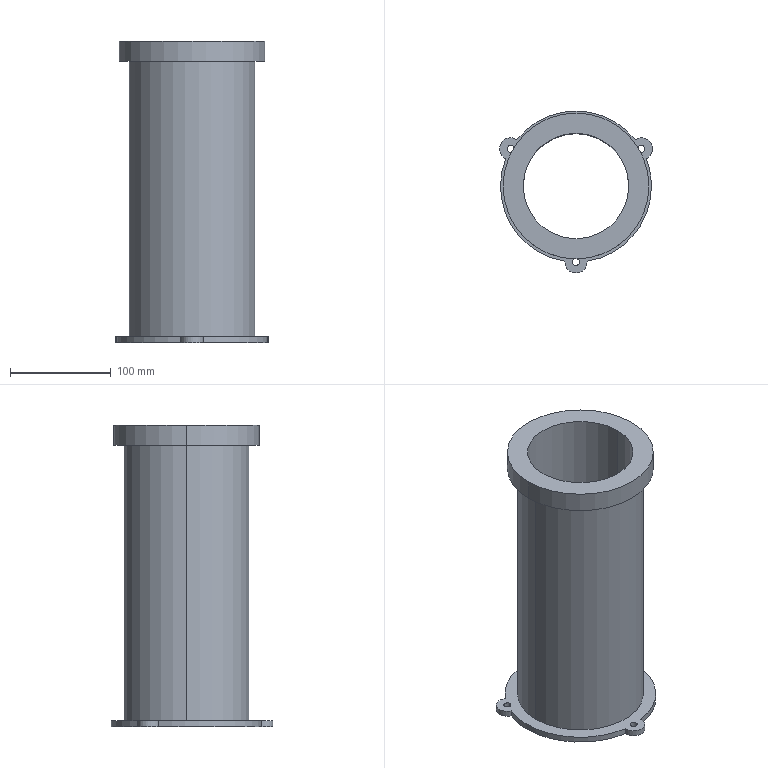Part | SolidWorks | features ICE 2, Extrusion 1 | 1 solid | 26 faces | box 151.904 x 161 x 300 mm | volume 1203905 mm3 | cylinder 22 | plane 4 | commonest cylinder face diameters 7 x6 22 x6 150 x4 105 x2 125 x2 145 x2
STEP:
#1=CARTESIAN_POINT('',(-61.452,37.5,-6.));
#2=VERTEX_POINT('',#1);
#3=CARTESIAN_POINT('',(-68.452,37.5,-6.));
#4=VERTEX_POINT('',#3);
#5=CARTESIAN_POINT('',(-64.952,37.5,-6.));
#6=DIRECTION('',(0.,0.,-1.));
#7=DIRECTION('',(-1.,0.,0.));
#8=AXIS2_PLACEMENT_3D('',#5,#6,#7);
#9=CIRCLE('',#8,3.5);
#10=EDGE_CURVE('',#2,#4,#9,.T.);
#11=ORIENTED_EDGE('',*,*,#10,.T.);
#12=CARTESIAN_POINT('',(-68.452,37.5,0.));
#13=VERTEX_POINT('',#12);
#14=CARTESIAN_POINT('',(-68.452,37.5,-6.));
#15=DIRECTION('',(0.,0.,1.));
#16=VECTOR('',#15,1000.);
#17=LINE('',#14,#16);
#18=EDGE_CURVE('',#4,#13,#17,.T.);
#19=ORIENTED_EDGE('',*,*,#18,.T.);
#20=CARTESIAN_POINT('',(-61.452,37.5,0.));
#21=VERTEX_POINT('',#20);
#22=CARTESIAN_POINT('',(-64.952,37.5,0.));
#23=DIRECTION('',(0.,0.,-1.));
#24=DIRECTION('',(-1.,0.,0.));
#25=AXIS2_PLACEMENT_3D('',#22,#23,#24);
#26=CIRCLE('',#25,3.5);
#27=EDGE_CURVE('',#21,#13,#26,.T.);
#28=ORIENTED_EDGE('',*,*,#27,.F.);
#29=CARTESIAN_POINT('',(-61.452,37.5,-6.));
#30=DIRECTION('',(0.,0.,1.));
#31=VECTOR('',#30,1000.);
#32=LINE('',#29,#31);
#33=EDGE_CURVE('',#2,#21,#32,.T.);
#34=ORIENTED_EDGE('',*,*,#33,.F.);
#35=EDGE_LOOP('',(#11,#19,#28,#34));
#36=FACE_OUTER_BOUND('',#35,.T.);
#37=CARTESIAN_POINT('',(-64.952,37.5,-6.));
#38=DIRECTION('',(0.,0.,1.));
#39=DIRECTION('',(1.,0.,0.));
#40=AXIS2_PLACEMENT_3D('',#37,#38,#39);
#41=CYLINDRICAL_SURFACE('',#40,3.5);
#42=ADVANCED_FACE('',(#36),#41,.F.);
#43=CARTESIAN_POINT('',(68.452,37.5,-6.));
#44=VERTEX_POINT('',#43);
#45=CARTESIAN_POINT('',(61.452,37.5,-6.));
#46=VERTEX_POINT('',#45);
#47=CARTESIAN_POINT('',(64.952,37.5,-6.));
#48=DIRECTION('',(0.,0.,-1.));
#49=DIRECTION('',(-1.,0.,0.));
#50=AXIS2_PLACEMENT_3D('',#47,#48,#49);
#51=CIRCLE('',#50,3.5);
#52=EDGE_CURVE('',#44,#46,#51,.T.);
#53=ORIENTED_EDGE('',*,*,#52,.T.);
#54=CARTESIAN_POINT('',(61.452,37.5,0.));
#55=VERTEX_POINT('',#54);
#56=CARTESIAN_POINT('',(61.452,37.5,-6.));
#57=DIRECTION('',(0.,0.,1.));
#58=VECTOR('',#57,1000.);
#59=LINE('',#56,#58);
#60=EDGE_CURVE('',#46,#55,#59,.T.);
#61=ORIENTED_EDGE('',*,*,#60,.T.);
#62=CARTESIAN_POINT('',(68.452,37.5,0.));
#63=VERTEX_POINT('',#62);
#64=CARTESIAN_POINT('',(64.952,37.5,0.));
#65=DIRECTION('',(0.,0.,-1.));
#66=DIRECTION('',(-1.,0.,0.));
#67=AXIS2_PLACEMENT_3D('',#64,#65,#66);
#68=CIRCLE('',#67,3.5);
#69=EDGE_CURVE('',#63,#55,#68,.T.);
#70=ORIENTED_EDGE('',*,*,#69,.F.);
#71=CARTESIAN_POINT('',(68.452,37.5,-6.));
#72=DIRECTION('',(0.,0.,1.));
#73=VECTOR('',#72,1000.);
#74=LINE('',#71,#73);
#75=EDGE_CURVE('',#44,#63,#74,.T.);
#76=ORIENTED_EDGE('',*,*,#75,.F.);
#77=EDGE_LOOP('',(#53,#61,#70,#76));
#78=FACE_OUTER_BOUND('',#77,.T.);
#79=CARTESIAN_POINT('',(64.952,37.5,-6.));
#80=DIRECTION('',(0.,0.,1.));
#81=DIRECTION('',(1.,0.,0.));
#82=AXIS2_PLACEMENT_3D('',#79,#80,#81);
#83=CYLINDRICAL_SURFACE('',#82,3.5);
#84=ADVANCED_FACE('',(#78),#83,.F.);
#85=CARTESIAN_POINT('',(3.5,-75.,-6.));
#86=VERTEX_POINT('',#85);
#87=CARTESIAN_POINT('',(-3.5,-75.,-6.));
#88=VERTEX_POINT('',#87);
#89=CARTESIAN_POINT('',(0.,-75.,-6.));
#90=DIRECTION('',(0.,0.,-1.));
#91=DIRECTION('',(-1.,0.,0.));
#92=AXIS2_PLACEMENT_3D('',#89,#90,#91);
#93=CIRCLE('',#92,3.5);
#94=EDGE_CURVE('',#86,#88,#93,.T.);
#95=ORIENTED_EDGE('',*,*,#94,.T.);
#96=CARTESIAN_POINT('',(-3.5,-75.,0.));
#97=VERTEX_POINT('',#96);
#98=CARTESIAN_POINT('',(-3.5,-75.,-6.));
#99=DIRECTION('',(0.,0.,1.));
#100=VECTOR('',#99,1000.);
#101=LINE('',#98,#100);
#102=EDGE_CURVE('',#88,#97,#101,.T.);
#103=ORIENTED_EDGE('',*,*,#102,.T.);
#104=CARTESIAN_POINT('',(3.5,-75.,0.));
#105=VERTEX_POINT('',#104);
#106=CARTESIAN_POINT('',(0.,-75.,0.));
#107=DIRECTION('',(0.,0.,-1.));
#108=DIRECTION('',(-1.,0.,0.));
#109=AXIS2_PLACEMENT_3D('',#106,#107,#108);
#110=CIRCLE('',#109,3.5);
#111=EDGE_CURVE('',#105,#97,#110,.T.);
#112=ORIENTED_EDGE('',*,*,#111,.F.);
#113=CARTESIAN_POINT('',(3.5,-75.,-6.));
#114=DIRECTION('',(0.,0.,1.));
#115=VECTOR('',#114,1000.);
#116=LINE('',#113,#115);
#117=EDGE_CURVE('',#86,#105,#116,.T.);
#118=ORIENTED_EDGE('',*,*,#117,.F.);
#119=EDGE_LOOP('',(#95,#103,#112,#118));
#120=FACE_OUTER_BOUND('',#119,.T.);
#121=CARTESIAN_POINT('',(0.,-75.,-6.));
#122=DIRECTION('',(0.,0.,1.));
#123=DIRECTION('',(1.,0.,0.));
#124=AXIS2_PLACEMENT_3D('',#121,#122,#123);
#125=CYLINDRICAL_SURFACE('',#124,3.5);
#126=ADVANCED_FACE('',(#120),#125,.F.);
#127=CARTESIAN_POINT('',(75.,0.,-6.));
#128=VERTEX_POINT('',#127);
#129=CARTESIAN_POINT('',(10.97,-74.193,-6.));
#130=VERTEX_POINT('',#129);
#131=CARTESIAN_POINT('',(0.,0.,-6.));
#132=DIRECTION('',(0.,0.,-1.));
#133=DIRECTION('',(-1.,0.,0.));
#134=AXIS2_PLACEMENT_3D('',#131,#132,#133);
#135=CIRCLE('',#134,75.);
#136=EDGE_CURVE('',#128,#130,#135,.T.);
#137=ORIENTED_EDGE('',*,*,#136,.F.);
#138=CARTESIAN_POINT('',(75.,0.,0.));
#139=VERTEX_POINT('',#138);
#140=CARTESIAN_POINT('',(75.,0.,-6.));
#141=DIRECTION('',(0.,0.,1.));
#142=VECTOR('',#141,1000.);
#143=LINE('',#140,#142);
#144=EDGE_CURVE('',#128,#139,#143,.T.);
#145=ORIENTED_EDGE('',*,*,#144,.T.);
#146=CARTESIAN_POINT('',(10.97,-74.193,0.));
#147=VERTEX_POINT('',#146);
#148=CARTESIAN_POINT('',(0.,0.,0.));
#149=DIRECTION('',(0.,0.,-1.));
#150=DIRECTION('',(-1.,0.,0.));
#151=AXIS2_PLACEMENT_3D('',#148,#149,#150);
#152=CIRCLE('',#151,75.);
#153=EDGE_CURVE('',#139,#147,#152,.T.);
#154=ORIENTED_EDGE('',*,*,#153,.T.);
#155=CARTESIAN_POINT('',(10.97,-74.193,-6.));
#156=DIRECTION('',(0.,0.,1.));
#157=VECTOR('',#156,1000.);
#158=LINE('',#155,#157);
#159=EDGE_CURVE('',#130,#147,#158,.T.);
#160=ORIENTED_EDGE('',*,*,#159,.F.);
#161=EDGE_LOOP('',(#137,#145,#154,#160));
#162=FACE_OUTER_BOUND('',#161,.T.);
#163=CARTESIAN_POINT('',(0.,0.,-6.));
#164=DIRECTION('',(0.,0.,1.));
#165=DIRECTION('',(1.,0.,0.));
#166=AXIS2_PLACEMENT_3D('',#163,#164,#165);
#167=CYLINDRICAL_SURFACE('',#166,75.);
#168=ADVANCED_FACE('',(#162),#167,.T.);
#169=CARTESIAN_POINT('',(75.952,37.5,-6.));
#170=VERTEX_POINT('',#169);
#171=CARTESIAN_POINT('',(69.739,27.596,-6.));
#172=VERTEX_POINT('',#171);
#173=CARTESIAN_POINT('',(64.952,37.5,-6.));
#174=DIRECTION('',(0.,0.,-1.));
#175=DIRECTION('',(-1.,0.,0.));
#176=AXIS2_PLACEMENT_3D('',#173,#174,#175);
#177=CIRCLE('',#176,11.);
#178=EDGE_CURVE('',#170,#172,#177,.T.);
#179=ORIENTED_EDGE('',*,*,#178,.F.);
#180=CARTESIAN_POINT('',(75.952,37.5,0.));
#181=VERTEX_POINT('',#180);
#182=CARTESIAN_POINT('',(75.952,37.5,-6.));
#183=DIRECTION('',(0.,0.,1.));
#184=VECTOR('',#183,1000.);
#185=LINE('',#182,#184);
#186=EDGE_CURVE('',#170,#181,#185,.T.);
#187=ORIENTED_EDGE('',*,*,#186,.T.);
#188=CARTESIAN_POINT('',(69.739,27.596,0.));
#189=VERTEX_POINT('',#188);
#190=CARTESIAN_POINT('',(64.952,37.5,0.));
#191=DIRECTION('',(0.,0.,-1.));
#192=DIRECTION('',(-1.,0.,0.));
#193=AXIS2_PLACEMENT_3D('',#190,#191,#192);
#194=CIRCLE('',#193,11.);
#195=EDGE_CURVE('',#181,#189,#194,.T.);
#196=ORIENTED_EDGE('',*,*,#195,.T.);
#197=CARTESIAN_POINT('',(69.739,27.596,-6.));
#198=DIRECTION('',(0.,0.,1.));
#199=VECTOR('',#198,1000.);
#200=LINE('',#197,#199);
#201=EDGE_CURVE('',#172,#189,#200,.T.);
#202=ORIENTED_EDGE('',*,*,#201,.F.);
#203=EDGE_LOOP('',(#179,#187,#196,#202));
#204=FACE_OUTER_BOUND('',#203,.T.);
#205=CARTESIAN_POINT('',(64.952,37.5,-6.));
#206=DIRECTION('',(0.,0.,1.));
#207=DIRECTION('',(1.,0.,0.));
#208=AXIS2_PLACEMENT_3D('',#205,#206,#207);
#209=CYLINDRICAL_SURFACE('',#208,11.);
#210=ADVANCED_FACE('',(#204),#209,.T.);
#211=CARTESIAN_POINT('',(-11.,-75.,-6.));
#212=VERTEX_POINT('',#211);
#213=CARTESIAN_POINT('',(-10.97,-74.193,-6.));
#214=VERTEX_POINT('',#213);
#215=CARTESIAN_POINT('',(0.,-75.,-6.));
#216=DIRECTION('',(0.,0.,-1.));
#217=DIRECTION('',(-1.,0.,0.));
#218=AXIS2_PLACEMENT_3D('',#215,#216,#217);
#219=CIRCLE('',#218,11.);
#220=EDGE_CURVE('',#212,#214,#219,.T.);
#221=ORIENTED_EDGE('',*,*,#220,.F.);
#222=CARTESIAN_POINT('',(-11.,-75.,0.));
#223=VERTEX_POINT('',#222);
#224=CARTESIAN_POINT('',(-11.,-75.,-6.));
#225=DIRECTION('',(0.,0.,1.));
#226=VECTOR('',#225,1000.);
#227=LINE('',#224,#226);
#228=EDGE_CURVE('',#212,#223,#227,.T.);
#229=ORIENTED_EDGE('',*,*,#228,.T.);
#230=CARTESIAN_POINT('',(-10.97,-74.193,0.));
#231=VERTEX_POINT('',#230);
#232=CARTESIAN_POINT('',(0.,-75.,0.));
#233=DIRECTION('',(0.,0.,-1.));
#234=DIRECTION('',(-1.,0.,0.));
#235=AXIS2_PLACEMENT_3D('',#232,#233,#234);
#236=CIRCLE('',#235,11.);
#237=EDGE_CURVE('',#223,#231,#236,.T.);
#238=ORIENTED_EDGE('',*,*,#237,.T.);
#239=CARTESIAN_POINT('',(-10.97,-74.193,-6.));
#240=DIRECTION('',(0.,0.,1.));
#241=VECTOR('',#240,1000.);
#242=LINE('',#239,#241);
#243=EDGE_CURVE('',#214,#231,#242,.T.);
#244=ORIENTED_EDGE('',*,*,#243,.F.);
#245=EDGE_LOOP('',(#221,#229,#238,#244));
#246=FACE_OUTER_BOUND('',#245,.T.);
#247=CARTESIAN_POINT('',(0.,-75.,-6.));
#248=DIRECTION('',(0.,0.,1.));
#249=DIRECTION('',(1.,0.,0.));
#250=AXIS2_PLACEMENT_3D('',#247,#248,#249);
#251=CYLINDRICAL_SURFACE('',#250,11.);
#252=ADVANCED_FACE('',(#246),#251,.T.);
#253=ORIENTED_EDGE('',*,*,#228,.F.);
#254=CARTESIAN_POINT('',(11.,-75.,-6.));
#255=VERTEX_POINT('',#254);
#256=CARTESIAN_POINT('',(0.,-75.,-6.));
#257=DIRECTION('',(0.,0.,-1.));
#258=DIRECTION('',(-1.,0.,0.));
#259=AXIS2_PLACEMENT_3D('',#256,#257,#258);
#260=CIRCLE('',#259,11.);
#261=EDGE_CURVE('',#255,#212,#260,.T.);
#262=ORIENTED_EDGE('',*,*,#261,.F.);
#263=CARTESIAN_POINT('',(11.,-75.,0.));
#264=VERTEX_POINT('',#263);
#265=CARTESIAN_POINT('',(11.,-75.,-6.));
#266=DIRECTION('',(0.,0.,1.));
#267=VECTOR('',#266,1000.);
#268=LINE('',#265,#267);
#269=EDGE_CURVE('',#255,#264,#268,.T.);
#270=ORIENTED_EDGE('',*,*,#269,.T.);
#271=CARTESIAN_POINT('',(0.,-75.,0.));
#272=DIRECTION('',(0.,0.,-1.));
#273=DIRECTION('',(-1.,0.,0.));
#274=AXIS2_PLACEMENT_3D('',#271,#272,#273);
#275=CIRCLE('',#274,11.);
#276=EDGE_CURVE('',#264,#223,#275,.T.);
#277=ORIENTED_EDGE('',*,*,#276,.T.);
#278=EDGE_LOOP('',(#253,#262,#270,#277));
#279=FACE_OUTER_BOUND('',#278,.T.);
#280=CARTESIAN_POINT('',(0.,-75.,-6.));
#281=DIRECTION('',(0.,0.,1.));
#282=DIRECTION('',(1.,0.,0.));
#283=AXIS2_PLACEMENT_3D('',#280,#281,#282);
#284=CYLINDRICAL_SURFACE('',#283,11.);
#285=ADVANCED_FACE('',(#279),#284,.T.);
#286=CARTESIAN_POINT('',(72.5,0.,294.));
#287=VERTEX_POINT('',#286);
#288=CARTESIAN_POINT('',(-72.5,0.,294.));
#289=VERTEX_POINT('',#288);
#290=CARTESIAN_POINT('',(0.,0.,294.));
#291=DIRECTION('',(0.,0.,1.));
#292=DIRECTION('',(1.,0.,0.));
#293=AXIS2_PLACEMENT_3D('',#290,#291,#292);
#294=CIRCLE('',#293,72.5);
#295=EDGE_CURVE('',#287,#289,#294,.T.);
#296=ORIENTED_EDGE('',*,*,#295,.F.);
#297=CARTESIAN_POINT('',(72.5,0.,274.));
#298=VERTEX_POINT('',#297);
#299=CARTESIAN_POINT('',(72.5,0.,294.));
#300=DIRECTION('',(0.,0.,-1.));
#301=VECTOR('',#300,1000.);
#302=LINE('',#299,#301);
#303=EDGE_CURVE('',#287,#298,#302,.T.);
#304=ORIENTED_EDGE('',*,*,#303,.T.);
#305=CARTESIAN_POINT('',(-72.5,0.,274.));
#306=VERTEX_POINT('',#305);
#307=CARTESIAN_POINT('',(0.,0.,274.));
#308=DIRECTION('',(0.,0.,1.));
#309=DIRECTION('',(1.,0.,0.));
#310=AXIS2_PLACEMENT_3D('',#307,#308,#309);
#311=CIRCLE('',#310,72.5);
#312=EDGE_CURVE('',#298,#306,#311,.T.);
#313=ORIENTED_EDGE('',*,*,#312,.T.);
#314=CARTESIAN_POINT('',(-72.5,0.,294.));
#315=DIRECTION('',(0.,0.,-1.));
#316=VECTOR('',#315,1000.);
#317=LINE('',#314,#316);
#318=EDGE_CURVE('',#289,#306,#317,.T.);
#319=ORIENTED_EDGE('',*,*,#318,.F.);
#320=EDGE_LOOP('',(#296,#304,#313,#319));
#321=FACE_OUTER_BOUND('',#320,.T.);
#322=CARTESIAN_POINT('',(0.,0.,294.));
#323=DIRECTION('',(0.,0.,-1.));
#324=DIRECTION('',(-1.,0.,0.));
#325=AXIS2_PLACEMENT_3D('',#322,#323,#324);
#326=CYLINDRICAL_SURFACE('',#325,72.5);
#327=ADVANCED_FACE('',(#321),#326,.T.);
#328=CARTESIAN_POINT('',(-52.5,0.,294.));
#329=VERTEX_POINT('',#328);
#330=CARTESIAN_POINT('',(52.5,0.,294.));
#331=VERTEX_POINT('',#330);
#332=CARTESIAN_POINT('',(0.,0.,294.));
#333=DIRECTION('',(0.,0.,1.));
#334=DIRECTION('',(1.,0.,0.));
#335=AXIS2_PLACEMENT_3D('',#332,#333,#334);
#336=CIRCLE('',#335,52.5);
#337=EDGE_CURVE('',#329,#331,#336,.T.);
#338=ORIENTED_EDGE('',*,*,#337,.T.);
#339=CARTESIAN_POINT('',(52.5,0.,-6.));
#340=VERTEX_POINT('',#339);
#341=CARTESIAN_POINT('',(52.5,0.,284.));
#342=DIRECTION('',(0.,0.,-1.));
#343=VECTOR('',#342,1000.);
#344=LINE('',#341,#343);
#345=EDGE_CURVE('',#331,#340,#344,.T.);
#346=ORIENTED_EDGE('',*,*,#345,.T.);
#347=CARTESIAN_POINT('',(-52.5,0.,-6.));
#348=VERTEX_POINT('',#347);
#349=CARTESIAN_POINT('',(0.,0.,-6.));
#350=DIRECTION('',(0.,0.,-1.));
#351=DIRECTION('',(-1.,0.,0.));
#352=AXIS2_PLACEMENT_3D('',#349,#350,#351);
#353=CIRCLE('',#352,52.5);
#354=EDGE_CURVE('',#340,#348,#353,.T.);
#355=ORIENTED_EDGE('',*,*,#354,.T.);
#356=CARTESIAN_POINT('',(-52.5,0.,284.));
#357=DIRECTION('',(0.,0.,-1.));
#358=VECTOR('',#357,1000.);
#359=LINE('',#356,#358);
#360=EDGE_CURVE('',#329,#348,#359,.T.);
#361=ORIENTED_EDGE('',*,*,#360,.F.);
#362=EDGE_LOOP('',(#338,#346,#355,#361));
#363=FACE_OUTER_BOUND('',#362,.T.);
#364=CARTESIAN_POINT('',(0.,0.,284.));
#365=DIRECTION('',(0.,0.,-1.));
#366=DIRECTION('',(-1.,0.,0.));
#367=AXIS2_PLACEMENT_3D('',#364,#365,#366);
#368=CYLINDRICAL_SURFACE('',#367,52.5);
#369=ADVANCED_FACE('',(#363),#368,.F.);
#370=CARTESIAN_POINT('',(62.5,0.,274.));
#371=VERTEX_POINT('',#370);
#372=CARTESIAN_POINT('',(-62.5,0.,274.));
#373=VERTEX_POINT('',#372);
#374=CARTESIAN_POINT('',(0.,0.,274.));
#375=DIRECTION('',(0.,0.,1.));
#376=DIRECTION('',(1.,0.,0.));
#377=AXIS2_PLACEMENT_3D('',#374,#375,#376);
#378=CIRCLE('',#377,62.5);
#379=EDGE_CURVE('',#371,#373,#378,.T.);
#380=ORIENTED_EDGE('',*,*,#379,.F.);
#381=CARTESIAN_POINT('',(62.5,0.,0.));
#382=VERTEX_POINT('',#381);
#383=CARTESIAN_POINT('',(62.5,0.,284.));
#384=DIRECTION('',(0.,0.,-1.));
#385=VECTOR('',#384,1000.);
#386=LINE('',#383,#385);
#387=EDGE_CURVE('',#371,#382,#386,.T.);
#388=ORIENTED_EDGE('',*,*,#387,.T.);
#389=CARTESIAN_POINT('',(-62.5,0.,0.));
#390=VERTEX_POINT('',#389);
#391=CARTESIAN_POINT('',(0.,0.,0.));
#392=DIRECTION('',(0.,0.,-1.));
#393=DIRECTION('',(-1.,0.,0.));
#394=AXIS2_PLACEMENT_3D('',#391,#392,#393);
#395=CIRCLE('',#394,62.5);
#396=EDGE_CURVE('',#390,#382,#395,.T.);
#397=ORIENTED_EDGE('',*,*,#396,.F.);
#398=CARTESIAN_POINT('',(-62.5,0.,284.));
#399=DIRECTION('',(0.,0.,-1.));
#400=VECTOR('',#399,1000.);
#401=LINE('',#398,#400);
#402=EDGE_CURVE('',#373,#390,#401,.T.);
#403=ORIENTED_EDGE('',*,*,#402,.F.);
#404=EDGE_LOOP('',(#380,#388,#397,#403));
#405=FACE_OUTER_BOUND('',#404,.T.);
#406=CARTESIAN_POINT('',(0.,0.,284.));
#407=DIRECTION('',(0.,0.,-1.));
#408=DIRECTION('',(-1.,0.,0.));
#409=AXIS2_PLACEMENT_3D('',#406,#407,#408);
#410=CYLINDRICAL_SURFACE('',#409,62.5);
#411=ADVANCED_FACE('',(#405),#410,.T.);
#412=ORIENTED_EDGE('',*,*,#387,.F.);
#413=CARTESIAN_POINT('',(0.,0.,274.));
#414=DIRECTION('',(0.,0.,1.));
#415=DIRECTION('',(1.,0.,0.));
#416=AXIS2_PLACEMENT_3D('',#413,#414,#415);
#417=CIRCLE('',#416,62.5);
#418=EDGE_CURVE('',#373,#371,#417,.T.);
#419=ORIENTED_EDGE('',*,*,#418,.F.);
#420=ORIENTED_EDGE('',*,*,#402,.T.);
#421=CARTESIAN_POINT('',(0.,0.,0.));
#422=DIRECTION('',(0.,0.,-1.));
#423=DIRECTION('',(-1.,0.,0.));
#424=AXIS2_PLACEMENT_3D('',#421,#422,#423);
#425=CIRCLE('',#424,62.5);
#426=EDGE_CURVE('',#382,#390,#425,.T.);
#427=ORIENTED_EDGE('',*,*,#426,.F.);
#428=EDGE_LOOP('',(#412,#419,#420,#427));
#429=FACE_OUTER_BOUND('',#428,.T.);
#430=CARTESIAN_POINT('',(0.,0.,284.));
#431=DIRECTION('',(0.,0.,-1.));
#432=DIRECTION('',(-1.,0.,0.));
#433=AXIS2_PLACEMENT_3D('',#430,#431,#432);
#434=CYLINDRICAL_SURFACE('',#433,62.5);
#435=ADVANCED_FACE('',(#429),#434,.T.);
#436=ORIENTED_EDGE('',*,*,#345,.F.);
#437=CARTESIAN_POINT('',(0.,0.,294.));
#438=DIRECTION('',(0.,0.,1.));
#439=DIRECTION('',(1.,0.,0.));
#440=AXIS2_PLACEMENT_3D('',#437,#438,#439);
#441=CIRCLE('',#440,52.5);
#442=EDGE_CURVE('',#331,#329,#441,.T.);
#443=ORIENTED_EDGE('',*,*,#442,.T.);
#444=ORIENTED_EDGE('',*,*,#360,.T.);
#445=CARTESIAN_POINT('',(0.,0.,-6.));
#446=DIRECTION('',(0.,0.,-1.));
#447=DIRECTION('',(-1.,0.,0.));
#448=AXIS2_PLACEMENT_3D('',#445,#446,#447);
#449=CIRCLE('',#448,52.5);
#450=EDGE_CURVE('',#348,#340,#449,.T.);
#451=ORIENTED_EDGE('',*,*,#450,.T.);
#452=EDGE_LOOP('',(#436,#443,#444,#451));
#453=FACE_OUTER_BOUND('',#452,.T.);
#454=CARTESIAN_POINT('',(0.,0.,284.));
#455=DIRECTION('',(0.,0.,-1.));
#456=DIRECTION('',(-1.,0.,0.));
#457=AXIS2_PLACEMENT_3D('',#454,#455,#456);
#458=CYLINDRICAL_SURFACE('',#457,52.5);
#459=ADVANCED_FACE('',(#453),#458,.F.);
#460=CARTESIAN_POINT('',(0.,0.,274.));
#461=DIRECTION('',(0.,0.,1.));
#462=DIRECTION('',(1.,0.,0.));
#463=AXIS2_PLACEMENT_3D('',#460,#461,#462);
#464=CIRCLE('',#463,72.5);
#465=EDGE_CURVE('',#306,#298,#464,.T.);
#466=ORIENTED_EDGE('',*,*,#465,.F.);
#467=ORIENTED_EDGE('',*,*,#312,.F.);
#468=EDGE_LOOP('',(#466,#467));
#469=FACE_OUTER_BOUND('',#468,.T.);
#470=ORIENTED_EDGE('',*,*,#418,.T.);
#471=ORIENTED_EDGE('',*,*,#379,.T.);
#472=EDGE_LOOP('',(#470,#471));
#473=FACE_BOUND('',#472,.T.);
#474=CARTESIAN_POINT('',(0.,0.,274.));
#475=DIRECTION('',(0.,0.,1.));
#476=DIRECTION('',(1.,0.,0.));
#477=AXIS2_PLACEMENT_3D('',#474,#475,#476);
#478=PLANE('',#477);
#479=ADVANCED_FACE('',(#469,#473),#478,.F.);
#480=CARTESIAN_POINT('',(0.,0.,294.));
#481=DIRECTION('',(0.,0.,1.));
#482=DIRECTION('',(1.,0.,0.));
#483=AXIS2_PLACEMENT_3D('',#480,#481,#482);
#484=CIRCLE('',#483,72.5);
#485=EDGE_CURVE('',#289,#287,#484,.T.);
#486=ORIENTED_EDGE('',*,*,#485,.T.);
#487=ORIENTED_EDGE('',*,*,#295,.T.);
#488=EDGE_LOOP('',(#486,#487));
#489=FACE_OUTER_BOUND('',#488,.T.);
#490=ORIENTED_EDGE('',*,*,#337,.F.);
#491=ORIENTED_EDGE('',*,*,#442,.F.);
#492=EDGE_LOOP('',(#490,#491));
#493=FACE_BOUND('',#492,.T.);
#494=CARTESIAN_POINT('',(0.,0.,294.));
#495=DIRECTION('',(0.,0.,1.));
#496=DIRECTION('',(1.,0.,0.));
#497=AXIS2_PLACEMENT_3D('',#494,#495,#496);
#498=PLANE('',#497);
#499=ADVANCED_FACE('',(#489,#493),#498,.T.);
#500=ORIENTED_EDGE('',*,*,#303,.F.);
#501=ORIENTED_EDGE('',*,*,#485,.F.);
#502=ORIENTED_EDGE('',*,*,#318,.T.);
#503=ORIENTED_EDGE('',*,*,#465,.T.);
#504=EDGE_LOOP('',(#500,#501,#502,#503));
#505=FACE_OUTER_BOUND('',#504,.T.);
#506=CARTESIAN_POINT('',(0.,0.,294.));
#507=DIRECTION('',(0.,0.,-1.));
#508=DIRECTION('',(-1.,0.,0.));
#509=AXIS2_PLACEMENT_3D('',#506,#507,#508);
#510=CYLINDRICAL_SURFACE('',#509,72.5);
#511=ADVANCED_FACE('',(#505),#510,.T.);
#512=ORIENTED_EDGE('',*,*,#27,.T.);
#513=CARTESIAN_POINT('',(-64.952,37.5,0.));
#514=DIRECTION('',(0.,0.,-1.));
#515=DIRECTION('',(-1.,0.,0.));
#516=AXIS2_PLACEMENT_3D('',#513,#514,#515);
#517=CIRCLE('',#516,3.5);
#518=EDGE_CURVE('',#13,#21,#517,.T.);
#519=ORIENTED_EDGE('',*,*,#518,.T.);
#520=EDGE_LOOP('',(#512,#519));
#521=FACE_BOUND('',#520,.T.);
#522=ORIENTED_EDGE('',*,*,#69,.T.);
#523=CARTESIAN_POINT('',(64.952,37.5,0.));
#524=DIRECTION('',(0.,0.,-1.));
#525=DIRECTION('',(-1.,0.,0.));
#526=AXIS2_PLACEMENT_3D('',#523,#524,#525);
#527=CIRCLE('',#526,3.5);
#528=EDGE_CURVE('',#55,#63,#527,.T.);
#529=ORIENTED_EDGE('',*,*,#528,.T.);
#530=EDGE_LOOP('',(#522,#529));
#531=FACE_BOUND('',#530,.T.);
#532=ORIENTED_EDGE('',*,*,#111,.T.);
#533=CARTESIAN_POINT('',(0.,-75.,0.));
#534=DIRECTION('',(0.,0.,-1.));
#535=DIRECTION('',(-1.,0.,0.));
#536=AXIS2_PLACEMENT_3D('',#533,#534,#535);
#537=CIRCLE('',#536,3.5);
#538=EDGE_CURVE('',#97,#105,#537,.T.);
#539=ORIENTED_EDGE('',*,*,#538,.T.);
#540=EDGE_LOOP('',(#532,#539));
#541=FACE_BOUND('',#540,.T.);
#542=CARTESIAN_POINT('',(0.,-75.,0.));
#543=DIRECTION('',(0.,0.,-1.));
#544=DIRECTION('',(-1.,0.,0.));
#545=AXIS2_PLACEMENT_3D('',#542,#543,#544);
#546=CIRCLE('',#545,11.);
#547=EDGE_CURVE('',#147,#264,#546,.T.);
#548=ORIENTED_EDGE('',*,*,#547,.F.);
#549=ORIENTED_EDGE('',*,*,#153,.F.);
#550=CARTESIAN_POINT('',(0.,0.,0.));
#551=DIRECTION('',(0.,0.,-1.));
#552=DIRECTION('',(-1.,0.,0.));
#553=AXIS2_PLACEMENT_3D('',#550,#551,#552);
#554=CIRCLE('',#553,75.);
#555=EDGE_CURVE('',#189,#139,#554,.T.);
#556=ORIENTED_EDGE('',*,*,#555,.F.);
#557=ORIENTED_EDGE('',*,*,#195,.F.);
#558=CARTESIAN_POINT('',(58.768,46.597,0.));
#559=VERTEX_POINT('',#558);
#560=CARTESIAN_POINT('',(64.952,37.5,0.));
#561=DIRECTION('',(0.,0.,-1.));
#562=DIRECTION('',(-1.,0.,0.));
#563=AXIS2_PLACEMENT_3D('',#560,#561,#562);
#564=CIRCLE('',#563,11.);
#565=EDGE_CURVE('',#559,#181,#564,.T.);
#566=ORIENTED_EDGE('',*,*,#565,.F.);
#567=CARTESIAN_POINT('',(-58.768,46.597,0.));
#568=VERTEX_POINT('',#567);
#569=CARTESIAN_POINT('',(0.,0.,0.));
#570=DIRECTION('',(0.,0.,-1.));
#571=DIRECTION('',(-1.,0.,0.));
#572=AXIS2_PLACEMENT_3D('',#569,#570,#571);
#573=CIRCLE('',#572,75.);
#574=EDGE_CURVE('',#568,#559,#573,.T.);
#575=ORIENTED_EDGE('',*,*,#574,.F.);
#576=CARTESIAN_POINT('',(-69.739,27.596,0.));
#577=VERTEX_POINT('',#576);
#578=CARTESIAN_POINT('',(-64.952,37.5,0.));
#579=DIRECTION('',(0.,0.,-1.));
#580=DIRECTION('',(-1.,0.,0.));
#581=AXIS2_PLACEMENT_3D('',#578,#579,#580);
#582=CIRCLE('',#581,11.);
#583=EDGE_CURVE('',#577,#568,#582,.T.);
#584=ORIENTED_EDGE('',*,*,#583,.F.);
#585=CARTESIAN_POINT('',(0.,0.,0.));
#586=DIRECTION('',(0.,0.,-1.));
#587=DIRECTION('',(-1.,0.,0.));
#588=AXIS2_PLACEMENT_3D('',#585,#586,#587);
#589=CIRCLE('',#588,75.);
#590=EDGE_CURVE('',#231,#577,#589,.T.);
#591=ORIENTED_EDGE('',*,*,#590,.F.);
#592=ORIENTED_EDGE('',*,*,#237,.F.);
#593=ORIENTED_EDGE('',*,*,#276,.F.);
#594=EDGE_LOOP('',(#548,#549,#556,#557,#566,#575,#584,#591,#592,#593));
#595=FACE_OUTER_BOUND('',#594,.T.);
#596=ORIENTED_EDGE('',*,*,#396,.T.);
#597=ORIENTED_EDGE('',*,*,#426,.T.);
#598=EDGE_LOOP('',(#596,#597));
#599=FACE_BOUND('',#598,.T.);
#600=CARTESIAN_POINT('',(0.,-37.5,0.));
#601=DIRECTION('',(0.,0.,-1.));
#602=DIRECTION('',(-1.,0.,0.));
#603=AXIS2_PLACEMENT_3D('',#600,#601,#602);
#604=PLANE('',#603);
#605=ADVANCED_FACE('',(#521,#531,#541,#595,#599),#604,.F.);
#606=ORIENTED_EDGE('',*,*,#52,.F.);
#607=CARTESIAN_POINT('',(64.952,37.5,-6.));
#608=DIRECTION('',(0.,0.,-1.));
#609=DIRECTION('',(-1.,0.,0.));
#610=AXIS2_PLACEMENT_3D('',#607,#608,#609);
#611=CIRCLE('',#610,3.5);
#612=EDGE_CURVE('',#46,#44,#611,.T.);
#613=ORIENTED_EDGE('',*,*,#612,.F.);
#614=EDGE_LOOP('',(#606,#613));
#615=FACE_BOUND('',#614,.T.);
#616=ORIENTED_EDGE('',*,*,#450,.F.);
#617=ORIENTED_EDGE('',*,*,#354,.F.);
#618=EDGE_LOOP('',(#616,#617));
#619=FACE_BOUND('',#618,.T.);
#620=CARTESIAN_POINT('',(0.,-75.,-6.));
#621=DIRECTION('',(0.,0.,-1.));
#622=DIRECTION('',(-1.,0.,0.));
#623=AXIS2_PLACEMENT_3D('',#620,#621,#622);
#624=CIRCLE('',#623,11.);
#625=EDGE_CURVE('',#130,#255,#624,.T.);
#626=ORIENTED_EDGE('',*,*,#625,.T.);
#627=ORIENTED_EDGE('',*,*,#261,.T.);
#628=ORIENTED_EDGE('',*,*,#220,.T.);
#629=CARTESIAN_POINT('',(-69.739,27.596,-6.));
#630=VERTEX_POINT('',#629);
#631=CARTESIAN_POINT('',(0.,0.,-6.));
#632=DIRECTION('',(0.,0.,-1.));
#633=DIRECTION('',(-1.,0.,0.));
#634=AXIS2_PLACEMENT_3D('',#631,#632,#633);
#635=CIRCLE('',#634,75.);
#636=EDGE_CURVE('',#214,#630,#635,.T.);
#637=ORIENTED_EDGE('',*,*,#636,.T.);
#638=CARTESIAN_POINT('',(-58.768,46.597,-6.));
#639=VERTEX_POINT('',#638);
#640=CARTESIAN_POINT('',(-64.952,37.5,-6.));
#641=DIRECTION('',(0.,0.,-1.));
#642=DIRECTION('',(-1.,0.,0.));
#643=AXIS2_PLACEMENT_3D('',#640,#641,#642);
#644=CIRCLE('',#643,11.);
#645=EDGE_CURVE('',#630,#639,#644,.T.);
#646=ORIENTED_EDGE('',*,*,#645,.T.);
#647=CARTESIAN_POINT('',(58.768,46.597,-6.));
#648=VERTEX_POINT('',#647);
#649=CARTESIAN_POINT('',(0.,0.,-6.));
#650=DIRECTION('',(0.,0.,-1.));
#651=DIRECTION('',(-1.,0.,0.));
#652=AXIS2_PLACEMENT_3D('',#649,#650,#651);
#653=CIRCLE('',#652,75.);
#654=EDGE_CURVE('',#639,#648,#653,.T.);
#655=ORIENTED_EDGE('',*,*,#654,.T.);
#656=CARTESIAN_POINT('',(64.952,37.5,-6.));
#657=DIRECTION('',(0.,0.,-1.));
#658=DIRECTION('',(-1.,0.,0.));
#659=AXIS2_PLACEMENT_3D('',#656,#657,#658);
#660=CIRCLE('',#659,11.);
#661=EDGE_CURVE('',#648,#170,#660,.T.);
#662=ORIENTED_EDGE('',*,*,#661,.T.);
#663=ORIENTED_EDGE('',*,*,#178,.T.);
#664=CARTESIAN_POINT('',(0.,0.,-6.));
#665=DIRECTION('',(0.,0.,-1.));
#666=DIRECTION('',(-1.,0.,0.));
#667=AXIS2_PLACEMENT_3D('',#664,#665,#666);
#668=CIRCLE('',#667,75.);
#669=EDGE_CURVE('',#172,#128,#668,.T.);
#670=ORIENTED_EDGE('',*,*,#669,.T.);
#671=ORIENTED_EDGE('',*,*,#136,.T.);
#672=EDGE_LOOP('',(#626,#627,#628,#637,#646,#655,#662,#663,#670,#671));
#673=FACE_OUTER_BOUND('',#672,.T.);
#674=ORIENTED_EDGE('',*,*,#94,.F.);
#675=CARTESIAN_POINT('',(0.,-75.,-6.));
#676=DIRECTION('',(0.,0.,-1.));
#677=DIRECTION('',(-1.,0.,0.));
#678=AXIS2_PLACEMENT_3D('',#675,#676,#677);
#679=CIRCLE('',#678,3.5);
#680=EDGE_CURVE('',#88,#86,#679,.T.);
#681=ORIENTED_EDGE('',*,*,#680,.F.);
#682=EDGE_LOOP('',(#674,#681));
#683=FACE_BOUND('',#682,.T.);
#684=ORIENTED_EDGE('',*,*,#10,.F.);
#685=CARTESIAN_POINT('',(-64.952,37.5,-6.));
#686=DIRECTION('',(0.,0.,-1.));
#687=DIRECTION('',(-1.,0.,0.));
#688=AXIS2_PLACEMENT_3D('',#685,#686,#687);
#689=CIRCLE('',#688,3.5);
#690=EDGE_CURVE('',#4,#2,#689,.T.);
#691=ORIENTED_EDGE('',*,*,#690,.F.);
#692=EDGE_LOOP('',(#684,#691));
#693=FACE_BOUND('',#692,.T.);
#694=CARTESIAN_POINT('',(0.,-37.5,-6.));
#695=DIRECTION('',(0.,0.,-1.));
#696=DIRECTION('',(-1.,0.,0.));
#697=AXIS2_PLACEMENT_3D('',#694,#695,#696);
#698=PLANE('',#697);
#699=ADVANCED_FACE('',(#615,#619,#673,#683,#693),#698,.T.);
#700=ORIENTED_EDGE('',*,*,#269,.F.);
#701=ORIENTED_EDGE('',*,*,#625,.F.);
#702=ORIENTED_EDGE('',*,*,#159,.T.);
#703=ORIENTED_EDGE('',*,*,#547,.T.);
#704=EDGE_LOOP('',(#700,#701,#702,#703));
#705=FACE_OUTER_BOUND('',#704,.T.);
#706=CARTESIAN_POINT('',(0.,-75.,-6.));
#707=DIRECTION('',(0.,0.,1.));
#708=DIRECTION('',(1.,0.,0.));
#709=AXIS2_PLACEMENT_3D('',#706,#707,#708);
#710=CYLINDRICAL_SURFACE('',#709,11.);
#711=ADVANCED_FACE('',(#705),#710,.T.);
#712=ORIENTED_EDGE('',*,*,#590,.T.);
#713=CARTESIAN_POINT('',(-69.739,27.596,-6.));
#714=DIRECTION('',(0.,0.,1.));
#715=VECTOR('',#714,1000.);
#716=LINE('',#713,#715);
#717=EDGE_CURVE('',#630,#577,#716,.T.);
#718=ORIENTED_EDGE('',*,*,#717,.F.);
#719=ORIENTED_EDGE('',*,*,#636,.F.);
#720=ORIENTED_EDGE('',*,*,#243,.T.);
#721=EDGE_LOOP('',(#712,#718,#719,#720));
#722=FACE_OUTER_BOUND('',#721,.T.);
#723=CARTESIAN_POINT('',(0.,0.,-6.));
#724=DIRECTION('',(0.,0.,1.));
#725=DIRECTION('',(1.,0.,0.));
#726=AXIS2_PLACEMENT_3D('',#723,#724,#725);
#727=CYLINDRICAL_SURFACE('',#726,75.);
#728=ADVANCED_FACE('',(#722),#727,.T.);
#729=ORIENTED_EDGE('',*,*,#583,.T.);
#730=CARTESIAN_POINT('',(-58.768,46.597,-6.));
#731=DIRECTION('',(0.,0.,1.));
#732=VECTOR('',#731,1000.);
#733=LINE('',#730,#732);
#734=EDGE_CURVE('',#639,#568,#733,.T.);
#735=ORIENTED_EDGE('',*,*,#734,.F.);
#736=ORIENTED_EDGE('',*,*,#645,.F.);
#737=ORIENTED_EDGE('',*,*,#717,.T.);
#738=EDGE_LOOP('',(#729,#735,#736,#737));
#739=FACE_OUTER_BOUND('',#738,.T.);
#740=CARTESIAN_POINT('',(-64.952,37.5,-6.));
#741=DIRECTION('',(0.,0.,1.));
#742=DIRECTION('',(1.,0.,0.));
#743=AXIS2_PLACEMENT_3D('',#740,#741,#742);
#744=CYLINDRICAL_SURFACE('',#743,11.);
#745=ADVANCED_FACE('',(#739),#744,.T.);
#746=ORIENTED_EDGE('',*,*,#574,.T.);
#747=CARTESIAN_POINT('',(58.768,46.597,-6.));
#748=DIRECTION('',(0.,0.,1.));
#749=VECTOR('',#748,1000.);
#750=LINE('',#747,#749);
#751=EDGE_CURVE('',#648,#559,#750,.T.);
#752=ORIENTED_EDGE('',*,*,#751,.F.);
#753=ORIENTED_EDGE('',*,*,#654,.F.);
#754=ORIENTED_EDGE('',*,*,#734,.T.);
#755=EDGE_LOOP('',(#746,#752,#753,#754));
#756=FACE_OUTER_BOUND('',#755,.T.);
#757=CARTESIAN_POINT('',(0.,0.,-6.));
#758=DIRECTION('',(0.,0.,1.));
#759=DIRECTION('',(1.,0.,0.));
#760=AXIS2_PLACEMENT_3D('',#757,#758,#759);
#761=CYLINDRICAL_SURFACE('',#760,75.);
#762=ADVANCED_FACE('',(#756),#761,.T.);
#763=ORIENTED_EDGE('',*,*,#186,.F.);
#764=ORIENTED_EDGE('',*,*,#661,.F.);
#765=ORIENTED_EDGE('',*,*,#751,.T.);
#766=ORIENTED_EDGE('',*,*,#565,.T.);
#767=EDGE_LOOP('',(#763,#764,#765,#766));
#768=FACE_OUTER_BOUND('',#767,.T.);
#769=CARTESIAN_POINT('',(64.952,37.5,-6.));
#770=DIRECTION('',(0.,0.,1.));
#771=DIRECTION('',(1.,0.,0.));
#772=AXIS2_PLACEMENT_3D('',#769,#770,#771);
#773=CYLINDRICAL_SURFACE('',#772,11.);
#774=ADVANCED_FACE('',(#768),#773,.T.);
#775=ORIENTED_EDGE('',*,*,#144,.F.);
#776=ORIENTED_EDGE('',*,*,#669,.F.);
#777=ORIENTED_EDGE('',*,*,#201,.T.);
#778=ORIENTED_EDGE('',*,*,#555,.T.);
#779=EDGE_LOOP('',(#775,#776,#777,#778));
#780=FACE_OUTER_BOUND('',#779,.T.);
#781=CARTESIAN_POINT('',(0.,0.,-6.));
#782=DIRECTION('',(0.,0.,1.));
#783=DIRECTION('',(1.,0.,0.));
#784=AXIS2_PLACEMENT_3D('',#781,#782,#783);
#785=CYLINDRICAL_SURFACE('',#784,75.);
#786=ADVANCED_FACE('',(#780),#785,.T.);
#787=ORIENTED_EDGE('',*,*,#102,.F.);
#788=ORIENTED_EDGE('',*,*,#680,.T.);
#789=ORIENTED_EDGE('',*,*,#117,.T.);
#790=ORIENTED_EDGE('',*,*,#538,.F.);
#791=EDGE_LOOP('',(#787,#788,#789,#790));
#792=FACE_OUTER_BOUND('',#791,.T.);
#793=CARTESIAN_POINT('',(0.,-75.,-6.));
#794=DIRECTION('',(0.,0.,1.));
#795=DIRECTION('',(1.,0.,0.));
#796=AXIS2_PLACEMENT_3D('',#793,#794,#795);
#797=CYLINDRICAL_SURFACE('',#796,3.5);
#798=ADVANCED_FACE('',(#792),#797,.F.);
#799=ORIENTED_EDGE('',*,*,#60,.F.);
#800=ORIENTED_EDGE('',*,*,#612,.T.);
#801=ORIENTED_EDGE('',*,*,#75,.T.);
#802=ORIENTED_EDGE('',*,*,#528,.F.);
#803=EDGE_LOOP('',(#799,#800,#801,#802));
#804=FACE_OUTER_BOUND('',#803,.T.);
#805=CARTESIAN_POINT('',(64.952,37.5,-6.));
#806=DIRECTION('',(0.,0.,1.));
#807=DIRECTION('',(1.,0.,0.));
#808=AXIS2_PLACEMENT_3D('',#805,#806,#807);
#809=CYLINDRICAL_SURFACE('',#808,3.5);
#810=ADVANCED_FACE('',(#804),#809,.F.);
#811=ORIENTED_EDGE('',*,*,#18,.F.);
#812=ORIENTED_EDGE('',*,*,#690,.T.);
#813=ORIENTED_EDGE('',*,*,#33,.T.);
#814=ORIENTED_EDGE('',*,*,#518,.F.);
#815=EDGE_LOOP('',(#811,#812,#813,#814));
#816=FACE_OUTER_BOUND('',#815,.T.);
#817=CARTESIAN_POINT('',(-64.952,37.5,-6.));
#818=DIRECTION('',(0.,0.,1.));
#819=DIRECTION('',(1.,0.,0.));
#820=AXIS2_PLACEMENT_3D('',#817,#818,#819);
#821=CYLINDRICAL_SURFACE('',#820,3.5);
#822=ADVANCED_FACE('',(#816),#821,.F.);
#823=CLOSED_SHELL('',(#42,#84,#126,#168,#210,#252,#285,#327,#369,#411,#435,#459,#479,#499,#511,#605,#699,#711,#728,#745,#762,#774,#786,#798,#810,#822));
#824=MANIFOLD_SOLID_BREP('',#823);
#825=CARTESIAN_POINT('',(0.,0.,0.));
#826=DIRECTION('',(0.,0.,1.));
#827=DIRECTION('',(1.,0.,0.));
#828=AXIS2_PLACEMENT_3D('',#825,#826,#827);
#829=(LENGTH_UNIT()NAMED_UNIT(*)SI_UNIT(.MILLI.,.METRE.));
#830=UNCERTAINTY_MEASURE_WITH_UNIT(LENGTH_MEASURE(0.00001),#829,'','');
#831=(NAMED_UNIT(*)PLANE_ANGLE_UNIT()SI_UNIT($,.RADIAN.));
#832=(NAMED_UNIT(*)SI_UNIT($,.STERADIAN.)SOLID_ANGLE_UNIT());
#833=(GEOMETRIC_REPRESENTATION_CONTEXT(3)GLOBAL_UNCERTAINTY_ASSIGNED_CONTEXT((#830))GLOBAL_UNIT_ASSIGNED_CONTEXT((#829,#831,#832))REPRESENTATION_CONTEXT('',''));
#834=ADVANCED_BREP_SHAPE_REPRESENTATION('',(#824,#828),#833);